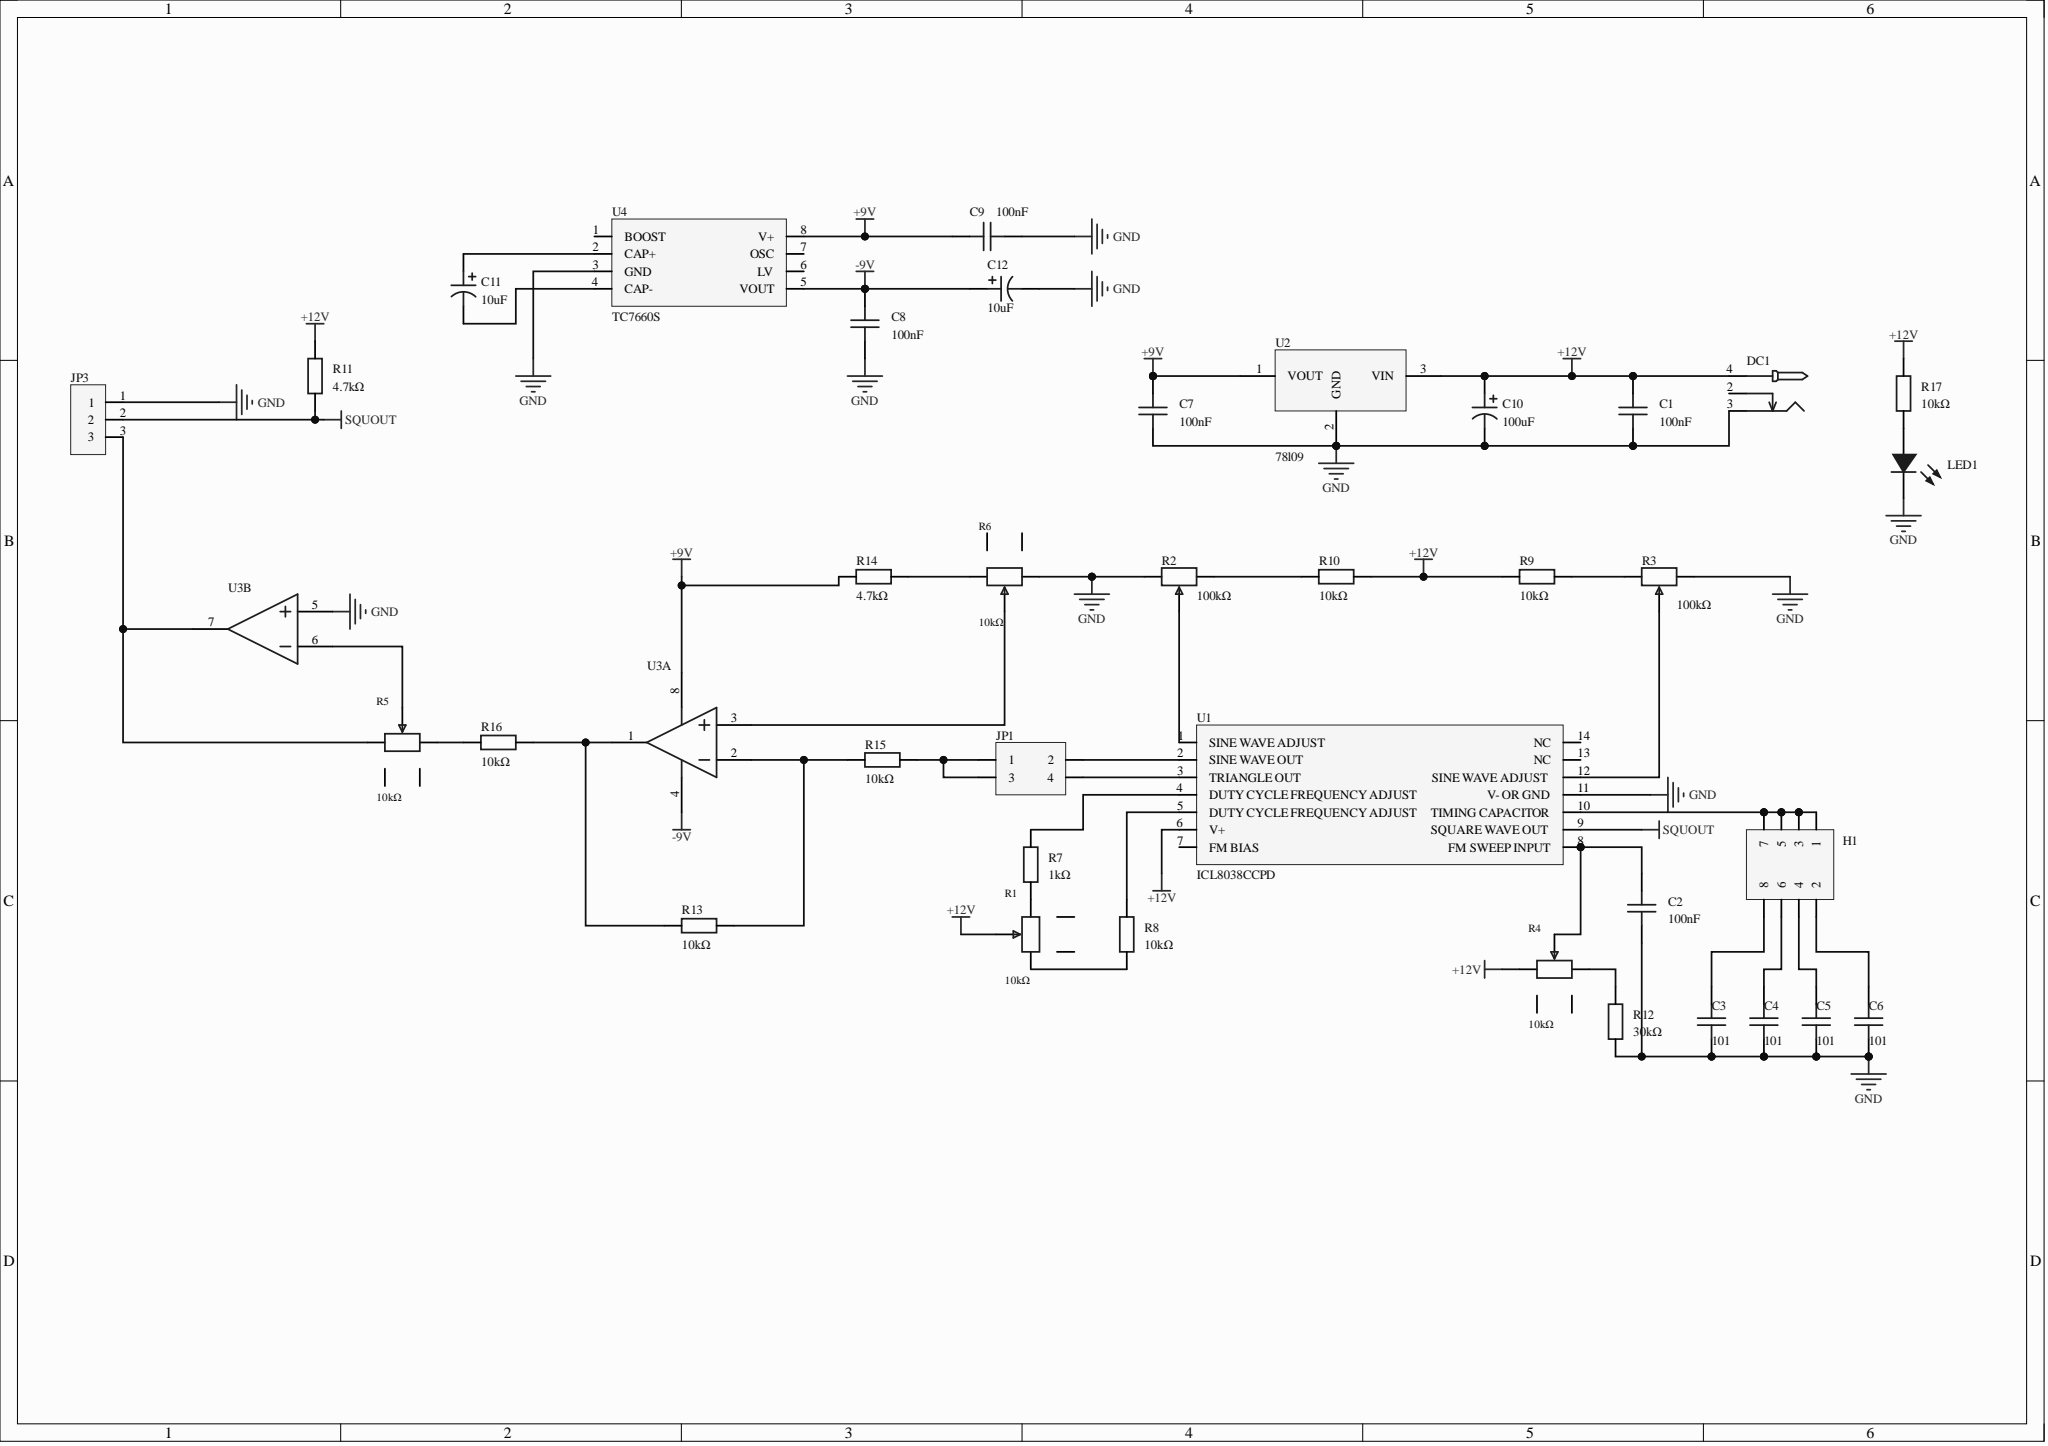Circuit board | Altium Designer | 38 parts | 33 nets
Bill of materials:
Comment,Description,Designator,Footprint,LibRef,Quantity
"100nF","Capacitance:100nF; tolerance:±10%; rated voltage:50V; temperature coefficient:X7R;","C1, C2, C7, C8, C9","CAP-TH_L5.1-W3.2-P5.08-D0.50","C323C104K5R5TA7301","5"
"101","Capacitance:100nF; tolerance:±10%; rated voltage:50V; temperature coefficient:X7R;","C3, C4, C5, C6","CAP-TH_L5.1-W3.2-P5.08-D0.50","C323C104K5R5TA7301","4"
"100uF","Capacitance:100uF; rated voltage:35V; ripple current:2.25A@100kHz; equivalent series resistance (ESR):38mΩ@100kHz; type:polymer;","C10","CAP-TH_BD6.3-P2.5-D0.6-FD-RYHG35V100UF","RYHG35V100UF6*8","1"
"10uF","Capacitance:10uF; tolerance:±20%; rated voltage:50V; ripple current:120mA@100KHz; equivalent series resistance (ESR):1.6Ω;","C11, C12","CAP-TH_BD5.0-P2.00-D0.8-FD-10UF50VC110GL","10UF50VC110GL","2"
"","","DC1","DC-2.0","DC-005_2.0","1"
"","","H1","HDR-TH_8P-P2.54-V-F-R2-C4-S2.54-1","HDR-F_2.54_2x4","1"
"","","JP1","HDR-TH_4P-P2.54-V-F-R2-C2-S2.54","HDR-F_2.54_2x2","1"
"","","JP3","CONN-TH_3P-P5.00_KF301-5.0-3P","HDR-M_2.54_1x3P","1"
"","","LED1","LED_TH-3mm","LED_TH-R_3mm","1"
"10kΩ","Resistance:100kΩ; tolerance:±10%; power:50mW;","R1, R4, R5, R6","RES-ADJ-TH_R09512N0-FB15A7.0-B103-005","R09592N0-AE4.5C3.0-B104-0007","4"
"100kΩ","Resistance:10kΩ; tolerance:±25%; power:100mW;","R2, R3","RES-ADJ-SMD_RM065-V1","RM065-103(10K)","2"
"1kΩ","","R7","Res_1/4W","Res_AXIAL-1/8W","1"
"10kΩ","","R8, R9, R10, R13, R15, R16, R17","Res_1/4W","Res_AXIAL-1/8W","7"
"4.7kΩ","","R11, R14","Res_1/4W","Res_AXIAL-1/8W","2"
"30kΩ","","R12","Res_1/4W","Res_AXIAL-1/8W","1"
"ICL8038CCPD","Interface type:-; max output frequency:-; output channels:4;","U1","PDIP-14_L19.2-W6.6-P2.54-LS7.6-BL","ICL8038CCPD_C5274778","1"
"78l09","","U2","TO-92-3_L4.5-W3.5-P1.27-L","78l09","1"
"","","U3","DIP-8_L9.3-W6.4-P2.54-LS7.6-TL","TL082","1"
"TC7660S","","U4","DIP-8_L10.0-W6.5-P2.54-LS7.6-BL","TC7660S","1"
Netlist (Protel format):
[
C1
CAP-TH_L5.1-W3.2-P5.08-D0.50
100nF



]
[
C2
CAP-TH_L5.1-W3.2-P5.08-D0.50
100nF



]
[
C3
CAP-TH_L5.1-W3.2-P5.08-D0.50
101



]
[
C4
CAP-TH_L5.1-W3.2-P5.08-D0.50
101



]
[
C5
CAP-TH_L5.1-W3.2-P5.08-D0.50
101



]
[
C6
CAP-TH_L5.1-W3.2-P5.08-D0.50
101



]
[
C7
CAP-TH_L5.1-W3.2-P5.08-D0.50
100nF



]
[
C8
CAP-TH_L5.1-W3.2-P5.08-D0.50
100nF



]
[
C9
CAP-TH_L5.1-W3.2-P5.08-D0.50
100nF



]
[
C10
CAP-TH_BD6.3-P2.5-D0.6-FD-RYHG35V100UF
100uF



]
[
C11
CAP-TH_BD5.0-P2.00-D0.8-FD-10UF50VC110GL
10uF



]
[
C12
CAP-TH_BD5.0-P2.00-D0.8-FD-10UF50VC110GL
10uF



]
[
DC1
DC-2.0




]
[
H1
HDR-TH_8P-P2.54-V-F-R2-C4-S2.54-1




]
[
JP1
HDR-TH_4P-P2.54-V-F-R2-C2-S2.54




]
[
JP3
CONN-TH_3P-P5.00_KF301-5.0-3P




]
[
LED1
LED_TH-3mm




]
[
R1
RES-ADJ-TH_R09512N0-FB15A7.0-B103-005
10kΩ



]
[
R2
RES-ADJ-SMD_RM065-V1
100kΩ



]
[
R3
RES-ADJ-SMD_RM065-V1
100kΩ



]
[
R4
RES-ADJ-TH_R09512N0-FB15A7.0-B103-005
10kΩ



]
[
R5
RES-ADJ-TH_R09512N0-FB15A7.0-B103-005
10kΩ



]
[
R6
RES-ADJ-TH_R09512N0-FB15A7.0-B103-005
10kΩ



]
[
R7
Res_1/4W
1kΩ



]
[
R8
Res_1/4W
10kΩ



]
[
R9
Res_1/4W
10kΩ



]
[
R10
Res_1/4W
10kΩ



]
[
R11
Res_1/4W
4.7kΩ



]
[
R12
Res_1/4W
30kΩ



]
[
R13
Res_1/4W
10kΩ



]
[
R14
Res_1/4W
4.7kΩ



]
[
R15
Res_1/4W
10kΩ



]
[
R16
Res_1/4W
10kΩ



]
[
R17
Res_1/4W
10kΩ



]
[
U1
PDIP-14_L19.2-W6.6-P2.54-LS7.6-BL
ICL8038CCPD



]
[
U2
TO-92-3_L4.5-W3.5-P1.27-L
78l09



]
[
U3
DIP-8_L9.3-W6.4-P2.54-LS7.6-TL




]
[
U4
DIP-8_L10.0-W6.5-P2.54-LS7.6-BL
TC7660S



]
(
SQUOUT
JP3-2
R11-1
U1-9
)
(
NetR13_2
R13-2
R15-1
U3-2
)
(
NetR13_1
R13-1
R16-2
U3-1
)
(
NetR8_2
R8-2
U1-5
)
(
NetR7_2
R7-2
U1-4
)
(
NetR6_2
R6-2
U3-3
)
(
NetR6_1
R6-1
R14-2
)
(
NetR5_2
R5-2
U3-6
)
(
NetR5_1
R5-1
R16-1
)
(
NetR4_1
R4-1
R12-2
)
(
NetR3_3
R3-3
R9-2
)
(
NetR3_2
R3-2
U1-12
)
(
NetR2_2
R2-2
U1-1
)
(
NetR2_1
R2-1
R10-1
)
(
NetR1_3
R1-3
R8-1
)
(
NetR1_1
R1-1
R7-1
)
(
NetLED1_1
LED1-1
R17-1
)
(
NetJP3_3
JP3-3
R5-3
U3-7
)
(
NetJP1_4
JP1-4
U1-3
)
(
NetJP1_2
JP1-2
U1-2
)
(
NetJP1_1
JP1-1
JP1-3
R15-2
)
(
NetH1_1
H1-1
H1-3
H1-5
H1-7
U1-10
)
(
NetC11_2
C11-2
U4-4
)
(
NetC11_1
C11-1
U4-2
)
(
NetC6_2
C6-2
H1-2
)
(
NetC5_2
C5-2
H1-4
)
(
NetC4_2
C4-2
H1-6
)
(
NetC3_2
C3-2
H1-8
)
(
NetC2_2
C2-2
R4-2
U1-8
)
(
GND
C1-1
C2-1
C3-1
C4-1
C5-1
C6-1
C7-1
C8-1
C9-1
C10-2
C12-2
DC1-3
JP3-1
LED1-2
R2-3
R3-1
R6-3
R12-1
U1-11
U2-2
U3-5
U4-3
)
(
-9V
C8-2
C12-1
U3-4
U4-5
)
(
+12V
C1-2
C10-1
DC1-4
R1-2
R4-3
R9-1
R10-2
R11-2
R17-2
U1-6
U2-3
)
(
+9V
C7-2
C9-2
R14-1
U2-1
U3-8
U4-8
)